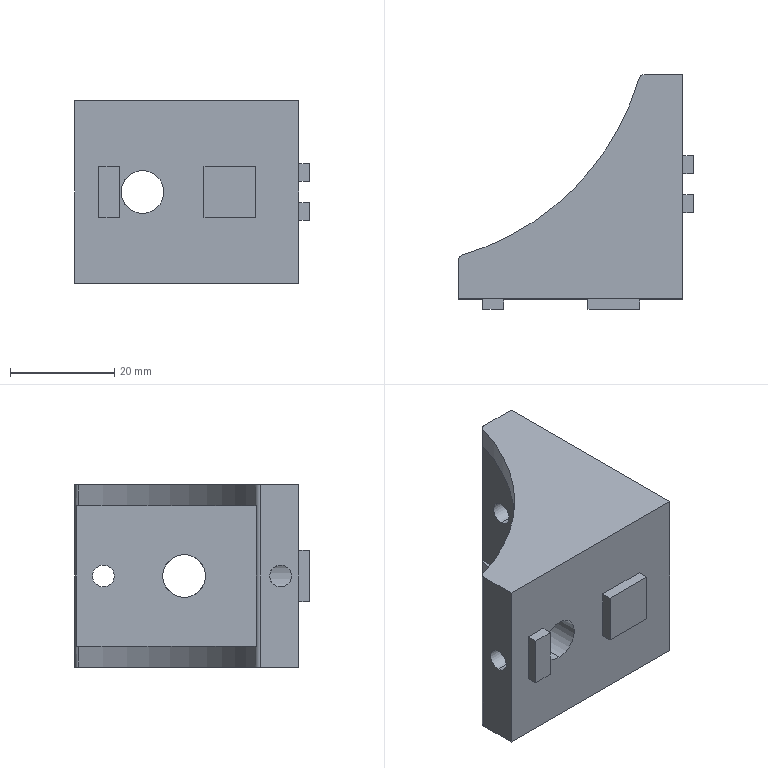Part | STEP file | HBLFSND8_45_HBLFSND8-45 | 1 solid | 52 faces | box 45 x 45 x 35 mm | volume 24695 mm3 | plane 40 | cylinder 12 | commonest cylinder face diameters 4.2 x4 8.2 x4 2 x2 100 x2